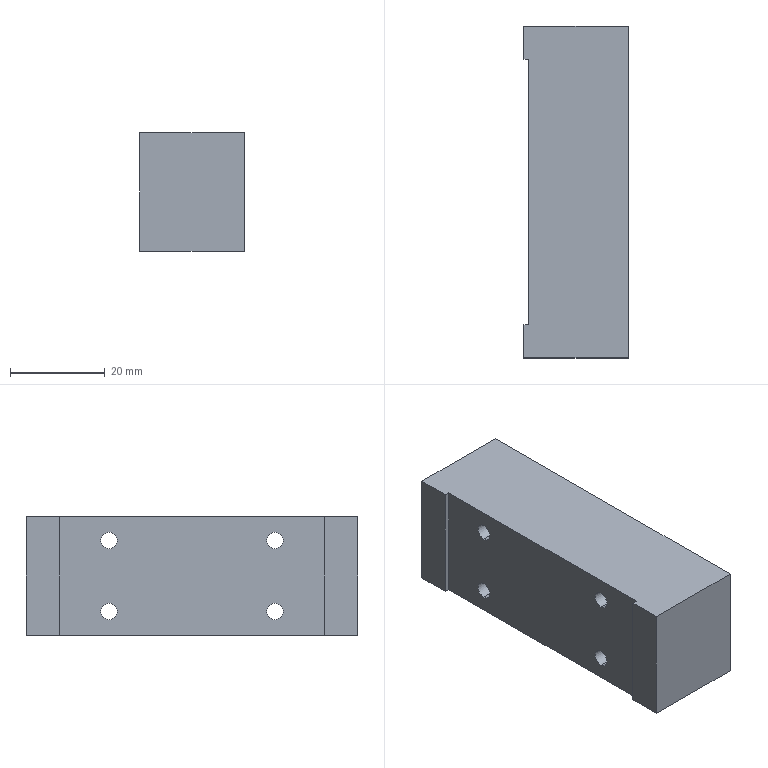Part | SolidWorks | features ICE 2, Extrusion 1 | 1 solid | 18 faces | box 22 x 70 x 25 mm | volume 36292 mm3 | plane 10 | cylinder 8 | commonest cylinder face diameters 3.5 x8
STEP:
#1=CARTESIAN_POINT('',(-10.,17.5,9.25));
#2=VERTEX_POINT('',#1);
#3=CARTESIAN_POINT('',(-10.,17.5,5.75));
#4=VERTEX_POINT('',#3);
#5=CARTESIAN_POINT('',(-10.,17.5,7.5));
#6=DIRECTION('',(1.,0.,0.));
#7=DIRECTION('',(0.,0.,1.));
#8=AXIS2_PLACEMENT_3D('',#5,#6,#7);
#9=CIRCLE('',#8,1.75);
#10=EDGE_CURVE('',#2,#4,#9,.T.);
#11=ORIENTED_EDGE('',*,*,#10,.F.);
#12=CARTESIAN_POINT('',(11.,17.5,9.25));
#13=VERTEX_POINT('',#12);
#14=CARTESIAN_POINT('',(-11.,17.5,9.25));
#15=DIRECTION('',(1.,0.,0.));
#16=VECTOR('',#15,1000.);
#17=LINE('',#14,#16);
#18=EDGE_CURVE('',#2,#13,#17,.T.);
#19=ORIENTED_EDGE('',*,*,#18,.T.);
#20=CARTESIAN_POINT('',(11.,17.5,5.75));
#21=VERTEX_POINT('',#20);
#22=CARTESIAN_POINT('',(11.,17.5,7.5));
#23=DIRECTION('',(1.,0.,0.));
#24=DIRECTION('',(0.,0.,1.));
#25=AXIS2_PLACEMENT_3D('',#22,#23,#24);
#26=CIRCLE('',#25,1.75);
#27=EDGE_CURVE('',#13,#21,#26,.T.);
#28=ORIENTED_EDGE('',*,*,#27,.T.);
#29=CARTESIAN_POINT('',(-11.,17.5,5.75));
#30=DIRECTION('',(1.,0.,0.));
#31=VECTOR('',#30,1000.);
#32=LINE('',#29,#31);
#33=EDGE_CURVE('',#4,#21,#32,.T.);
#34=ORIENTED_EDGE('',*,*,#33,.F.);
#35=EDGE_LOOP('',(#11,#19,#28,#34));
#36=FACE_OUTER_BOUND('',#35,.T.);
#37=CARTESIAN_POINT('',(-11.,17.5,7.5));
#38=DIRECTION('',(1.,0.,0.));
#39=DIRECTION('',(0.,0.,-1.));
#40=AXIS2_PLACEMENT_3D('',#37,#38,#39);
#41=CYLINDRICAL_SURFACE('',#40,1.75);
#42=ADVANCED_FACE('',(#36),#41,.F.);
#43=CARTESIAN_POINT('',(-10.,17.5,-5.75));
#44=VERTEX_POINT('',#43);
#45=CARTESIAN_POINT('',(-10.,17.5,-9.25));
#46=VERTEX_POINT('',#45);
#47=CARTESIAN_POINT('',(-10.,17.5,-7.5));
#48=DIRECTION('',(1.,0.,0.));
#49=DIRECTION('',(0.,0.,1.));
#50=AXIS2_PLACEMENT_3D('',#47,#48,#49);
#51=CIRCLE('',#50,1.75);
#52=EDGE_CURVE('',#44,#46,#51,.T.);
#53=ORIENTED_EDGE('',*,*,#52,.F.);
#54=CARTESIAN_POINT('',(11.,17.5,-5.75));
#55=VERTEX_POINT('',#54);
#56=CARTESIAN_POINT('',(-11.,17.5,-5.75));
#57=DIRECTION('',(1.,0.,0.));
#58=VECTOR('',#57,1000.);
#59=LINE('',#56,#58);
#60=EDGE_CURVE('',#44,#55,#59,.T.);
#61=ORIENTED_EDGE('',*,*,#60,.T.);
#62=CARTESIAN_POINT('',(11.,17.5,-9.25));
#63=VERTEX_POINT('',#62);
#64=CARTESIAN_POINT('',(11.,17.5,-7.5));
#65=DIRECTION('',(1.,0.,0.));
#66=DIRECTION('',(0.,0.,-1.));
#67=AXIS2_PLACEMENT_3D('',#64,#65,#66);
#68=CIRCLE('',#67,1.75);
#69=EDGE_CURVE('',#55,#63,#68,.T.);
#70=ORIENTED_EDGE('',*,*,#69,.T.);
#71=CARTESIAN_POINT('',(-11.,17.5,-9.25));
#72=DIRECTION('',(1.,0.,0.));
#73=VECTOR('',#72,1000.);
#74=LINE('',#71,#73);
#75=EDGE_CURVE('',#46,#63,#74,.T.);
#76=ORIENTED_EDGE('',*,*,#75,.F.);
#77=EDGE_LOOP('',(#53,#61,#70,#76));
#78=FACE_OUTER_BOUND('',#77,.T.);
#79=CARTESIAN_POINT('',(-11.,17.5,-7.5));
#80=DIRECTION('',(1.,0.,0.));
#81=DIRECTION('',(0.,0.,-1.));
#82=AXIS2_PLACEMENT_3D('',#79,#80,#81);
#83=CYLINDRICAL_SURFACE('',#82,1.75);
#84=ADVANCED_FACE('',(#78),#83,.F.);
#85=CARTESIAN_POINT('',(-10.,52.5,-5.75));
#86=VERTEX_POINT('',#85);
#87=CARTESIAN_POINT('',(-10.,52.5,-9.25));
#88=VERTEX_POINT('',#87);
#89=CARTESIAN_POINT('',(-10.,52.5,-7.5));
#90=DIRECTION('',(1.,0.,0.));
#91=DIRECTION('',(0.,0.,1.));
#92=AXIS2_PLACEMENT_3D('',#89,#90,#91);
#93=CIRCLE('',#92,1.75);
#94=EDGE_CURVE('',#86,#88,#93,.T.);
#95=ORIENTED_EDGE('',*,*,#94,.F.);
#96=CARTESIAN_POINT('',(11.,52.5,-5.75));
#97=VERTEX_POINT('',#96);
#98=CARTESIAN_POINT('',(-11.,52.5,-5.75));
#99=DIRECTION('',(1.,0.,0.));
#100=VECTOR('',#99,1000.);
#101=LINE('',#98,#100);
#102=EDGE_CURVE('',#86,#97,#101,.T.);
#103=ORIENTED_EDGE('',*,*,#102,.T.);
#104=CARTESIAN_POINT('',(11.,52.5,-9.25));
#105=VERTEX_POINT('',#104);
#106=CARTESIAN_POINT('',(11.,52.5,-7.5));
#107=DIRECTION('',(1.,0.,0.));
#108=DIRECTION('',(0.,0.,1.));
#109=AXIS2_PLACEMENT_3D('',#106,#107,#108);
#110=CIRCLE('',#109,1.75);
#111=EDGE_CURVE('',#97,#105,#110,.T.);
#112=ORIENTED_EDGE('',*,*,#111,.T.);
#113=CARTESIAN_POINT('',(-11.,52.5,-9.25));
#114=DIRECTION('',(1.,0.,0.));
#115=VECTOR('',#114,1000.);
#116=LINE('',#113,#115);
#117=EDGE_CURVE('',#88,#105,#116,.T.);
#118=ORIENTED_EDGE('',*,*,#117,.F.);
#119=EDGE_LOOP('',(#95,#103,#112,#118));
#120=FACE_OUTER_BOUND('',#119,.T.);
#121=CARTESIAN_POINT('',(-11.,52.5,-7.5));
#122=DIRECTION('',(1.,0.,0.));
#123=DIRECTION('',(0.,0.,-1.));
#124=AXIS2_PLACEMENT_3D('',#121,#122,#123);
#125=CYLINDRICAL_SURFACE('',#124,1.75);
#126=ADVANCED_FACE('',(#120),#125,.F.);
#127=CARTESIAN_POINT('',(-10.,52.5,9.25));
#128=VERTEX_POINT('',#127);
#129=CARTESIAN_POINT('',(-10.,52.5,5.75));
#130=VERTEX_POINT('',#129);
#131=CARTESIAN_POINT('',(-10.,52.5,7.5));
#132=DIRECTION('',(1.,0.,0.));
#133=DIRECTION('',(0.,0.,1.));
#134=AXIS2_PLACEMENT_3D('',#131,#132,#133);
#135=CIRCLE('',#134,1.75);
#136=EDGE_CURVE('',#128,#130,#135,.T.);
#137=ORIENTED_EDGE('',*,*,#136,.F.);
#138=CARTESIAN_POINT('',(11.,52.5,9.25));
#139=VERTEX_POINT('',#138);
#140=CARTESIAN_POINT('',(-11.,52.5,9.25));
#141=DIRECTION('',(1.,0.,0.));
#142=VECTOR('',#141,1000.);
#143=LINE('',#140,#142);
#144=EDGE_CURVE('',#128,#139,#143,.T.);
#145=ORIENTED_EDGE('',*,*,#144,.T.);
#146=CARTESIAN_POINT('',(11.,52.5,5.75));
#147=VERTEX_POINT('',#146);
#148=CARTESIAN_POINT('',(11.,52.5,7.5));
#149=DIRECTION('',(1.,0.,0.));
#150=DIRECTION('',(0.,0.,-1.));
#151=AXIS2_PLACEMENT_3D('',#148,#149,#150);
#152=CIRCLE('',#151,1.75);
#153=EDGE_CURVE('',#139,#147,#152,.T.);
#154=ORIENTED_EDGE('',*,*,#153,.T.);
#155=CARTESIAN_POINT('',(-11.,52.5,5.75));
#156=DIRECTION('',(1.,0.,0.));
#157=VECTOR('',#156,1000.);
#158=LINE('',#155,#157);
#159=EDGE_CURVE('',#130,#147,#158,.T.);
#160=ORIENTED_EDGE('',*,*,#159,.F.);
#161=EDGE_LOOP('',(#137,#145,#154,#160));
#162=FACE_OUTER_BOUND('',#161,.T.);
#163=CARTESIAN_POINT('',(-11.,52.5,7.5));
#164=DIRECTION('',(1.,0.,0.));
#165=DIRECTION('',(0.,0.,-1.));
#166=AXIS2_PLACEMENT_3D('',#163,#164,#165);
#167=CYLINDRICAL_SURFACE('',#166,1.75);
#168=ADVANCED_FACE('',(#162),#167,.F.);
#169=CARTESIAN_POINT('',(-11.,7.,12.5));
#170=VERTEX_POINT('',#169);
#171=CARTESIAN_POINT('',(-11.,0.,12.5));
#172=VERTEX_POINT('',#171);
#173=CARTESIAN_POINT('',(-11.,70.,12.5));
#174=DIRECTION('',(0.,-1.,0.));
#175=VECTOR('',#174,1000.);
#176=LINE('',#173,#175);
#177=EDGE_CURVE('',#170,#172,#176,.T.);
#178=ORIENTED_EDGE('',*,*,#177,.F.);
#179=CARTESIAN_POINT('',(-11.,7.,-12.5));
#180=VERTEX_POINT('',#179);
#181=CARTESIAN_POINT('',(-11.,7.,-12.5));
#182=DIRECTION('',(0.,0.,1.));
#183=VECTOR('',#182,1000.);
#184=LINE('',#181,#183);
#185=EDGE_CURVE('',#180,#170,#184,.T.);
#186=ORIENTED_EDGE('',*,*,#185,.F.);
#187=CARTESIAN_POINT('',(-11.,0.,-12.5));
#188=VERTEX_POINT('',#187);
#189=CARTESIAN_POINT('',(-11.,70.,-12.5));
#190=DIRECTION('',(0.,-1.,0.));
#191=VECTOR('',#190,1000.);
#192=LINE('',#189,#191);
#193=EDGE_CURVE('',#180,#188,#192,.T.);
#194=ORIENTED_EDGE('',*,*,#193,.T.);
#195=CARTESIAN_POINT('',(-11.,0.,-12.5));
#196=DIRECTION('',(0.,0.,1.));
#197=VECTOR('',#196,1000.);
#198=LINE('',#195,#197);
#199=EDGE_CURVE('',#188,#172,#198,.T.);
#200=ORIENTED_EDGE('',*,*,#199,.T.);
#201=EDGE_LOOP('',(#178,#186,#194,#200));
#202=FACE_OUTER_BOUND('',#201,.T.);
#203=CARTESIAN_POINT('',(-11.,70.,-12.5));
#204=DIRECTION('',(1.,0.,0.));
#205=DIRECTION('',(0.,0.,-1.));
#206=AXIS2_PLACEMENT_3D('',#203,#204,#205);
#207=PLANE('',#206);
#208=ADVANCED_FACE('',(#202),#207,.F.);
#209=ORIENTED_EDGE('',*,*,#144,.F.);
#210=CARTESIAN_POINT('',(-10.,52.5,7.5));
#211=DIRECTION('',(1.,0.,0.));
#212=DIRECTION('',(0.,0.,1.));
#213=AXIS2_PLACEMENT_3D('',#210,#211,#212);
#214=CIRCLE('',#213,1.75);
#215=EDGE_CURVE('',#130,#128,#214,.T.);
#216=ORIENTED_EDGE('',*,*,#215,.F.);
#217=ORIENTED_EDGE('',*,*,#159,.T.);
#218=CARTESIAN_POINT('',(11.,52.5,7.5));
#219=DIRECTION('',(1.,0.,0.));
#220=DIRECTION('',(0.,0.,-1.));
#221=AXIS2_PLACEMENT_3D('',#218,#219,#220);
#222=CIRCLE('',#221,1.75);
#223=EDGE_CURVE('',#147,#139,#222,.T.);
#224=ORIENTED_EDGE('',*,*,#223,.T.);
#225=EDGE_LOOP('',(#209,#216,#217,#224));
#226=FACE_OUTER_BOUND('',#225,.T.);
#227=CARTESIAN_POINT('',(-11.,52.5,7.5));
#228=DIRECTION('',(1.,0.,0.));
#229=DIRECTION('',(0.,0.,-1.));
#230=AXIS2_PLACEMENT_3D('',#227,#228,#229);
#231=CYLINDRICAL_SURFACE('',#230,1.75);
#232=ADVANCED_FACE('',(#226),#231,.F.);
#233=ORIENTED_EDGE('',*,*,#102,.F.);
#234=CARTESIAN_POINT('',(-10.,52.5,-7.5));
#235=DIRECTION('',(1.,0.,0.));
#236=DIRECTION('',(0.,0.,1.));
#237=AXIS2_PLACEMENT_3D('',#234,#235,#236);
#238=CIRCLE('',#237,1.75);
#239=EDGE_CURVE('',#88,#86,#238,.T.);
#240=ORIENTED_EDGE('',*,*,#239,.F.);
#241=ORIENTED_EDGE('',*,*,#117,.T.);
#242=CARTESIAN_POINT('',(11.,52.5,-7.5));
#243=DIRECTION('',(1.,0.,0.));
#244=DIRECTION('',(0.,0.,1.));
#245=AXIS2_PLACEMENT_3D('',#242,#243,#244);
#246=CIRCLE('',#245,1.75);
#247=EDGE_CURVE('',#105,#97,#246,.T.);
#248=ORIENTED_EDGE('',*,*,#247,.T.);
#249=EDGE_LOOP('',(#233,#240,#241,#248));
#250=FACE_OUTER_BOUND('',#249,.T.);
#251=CARTESIAN_POINT('',(-11.,52.5,-7.5));
#252=DIRECTION('',(1.,0.,0.));
#253=DIRECTION('',(0.,0.,-1.));
#254=AXIS2_PLACEMENT_3D('',#251,#252,#253);
#255=CYLINDRICAL_SURFACE('',#254,1.75);
#256=ADVANCED_FACE('',(#250),#255,.F.);
#257=ORIENTED_EDGE('',*,*,#60,.F.);
#258=CARTESIAN_POINT('',(-10.,17.5,-7.5));
#259=DIRECTION('',(1.,0.,0.));
#260=DIRECTION('',(0.,0.,1.));
#261=AXIS2_PLACEMENT_3D('',#258,#259,#260);
#262=CIRCLE('',#261,1.75);
#263=EDGE_CURVE('',#46,#44,#262,.T.);
#264=ORIENTED_EDGE('',*,*,#263,.F.);
#265=ORIENTED_EDGE('',*,*,#75,.T.);
#266=CARTESIAN_POINT('',(11.,17.5,-7.5));
#267=DIRECTION('',(1.,0.,0.));
#268=DIRECTION('',(0.,0.,-1.));
#269=AXIS2_PLACEMENT_3D('',#266,#267,#268);
#270=CIRCLE('',#269,1.75);
#271=EDGE_CURVE('',#63,#55,#270,.T.);
#272=ORIENTED_EDGE('',*,*,#271,.T.);
#273=EDGE_LOOP('',(#257,#264,#265,#272));
#274=FACE_OUTER_BOUND('',#273,.T.);
#275=CARTESIAN_POINT('',(-11.,17.5,-7.5));
#276=DIRECTION('',(1.,0.,0.));
#277=DIRECTION('',(0.,0.,-1.));
#278=AXIS2_PLACEMENT_3D('',#275,#276,#277);
#279=CYLINDRICAL_SURFACE('',#278,1.75);
#280=ADVANCED_FACE('',(#274),#279,.F.);
#281=ORIENTED_EDGE('',*,*,#18,.F.);
#282=CARTESIAN_POINT('',(-10.,17.5,7.5));
#283=DIRECTION('',(1.,0.,0.));
#284=DIRECTION('',(0.,0.,1.));
#285=AXIS2_PLACEMENT_3D('',#282,#283,#284);
#286=CIRCLE('',#285,1.75);
#287=EDGE_CURVE('',#4,#2,#286,.T.);
#288=ORIENTED_EDGE('',*,*,#287,.F.);
#289=ORIENTED_EDGE('',*,*,#33,.T.);
#290=CARTESIAN_POINT('',(11.,17.5,7.5));
#291=DIRECTION('',(1.,0.,0.));
#292=DIRECTION('',(0.,0.,1.));
#293=AXIS2_PLACEMENT_3D('',#290,#291,#292);
#294=CIRCLE('',#293,1.75);
#295=EDGE_CURVE('',#21,#13,#294,.T.);
#296=ORIENTED_EDGE('',*,*,#295,.T.);
#297=EDGE_LOOP('',(#281,#288,#289,#296));
#298=FACE_OUTER_BOUND('',#297,.T.);
#299=CARTESIAN_POINT('',(-11.,17.5,7.5));
#300=DIRECTION('',(1.,0.,0.));
#301=DIRECTION('',(0.,0.,-1.));
#302=AXIS2_PLACEMENT_3D('',#299,#300,#301);
#303=CYLINDRICAL_SURFACE('',#302,1.75);
#304=ADVANCED_FACE('',(#298),#303,.F.);
#305=ORIENTED_EDGE('',*,*,#295,.F.);
#306=ORIENTED_EDGE('',*,*,#27,.F.);
#307=EDGE_LOOP('',(#305,#306));
#308=FACE_BOUND('',#307,.T.);
#309=ORIENTED_EDGE('',*,*,#271,.F.);
#310=ORIENTED_EDGE('',*,*,#69,.F.);
#311=EDGE_LOOP('',(#309,#310));
#312=FACE_BOUND('',#311,.T.);
#313=ORIENTED_EDGE('',*,*,#247,.F.);
#314=ORIENTED_EDGE('',*,*,#111,.F.);
#315=EDGE_LOOP('',(#313,#314));
#316=FACE_BOUND('',#315,.T.);
#317=ORIENTED_EDGE('',*,*,#223,.F.);
#318=ORIENTED_EDGE('',*,*,#153,.F.);
#319=EDGE_LOOP('',(#317,#318));
#320=FACE_BOUND('',#319,.T.);
#321=CARTESIAN_POINT('',(11.,0.,12.5));
#322=VERTEX_POINT('',#321);
#323=CARTESIAN_POINT('',(11.,0.,-12.5));
#324=VERTEX_POINT('',#323);
#325=CARTESIAN_POINT('',(11.,0.,-12.5));
#326=DIRECTION('',(0.,0.,-1.));
#327=VECTOR('',#326,1000.);
#328=LINE('',#325,#327);
#329=EDGE_CURVE('',#322,#324,#328,.T.);
#330=ORIENTED_EDGE('',*,*,#329,.T.);
#331=CARTESIAN_POINT('',(11.,70.,-12.5));
#332=VERTEX_POINT('',#331);
#333=CARTESIAN_POINT('',(11.,70.,-12.5));
#334=DIRECTION('',(0.,-1.,0.));
#335=VECTOR('',#334,1000.);
#336=LINE('',#333,#335);
#337=EDGE_CURVE('',#332,#324,#336,.T.);
#338=ORIENTED_EDGE('',*,*,#337,.F.);
#339=CARTESIAN_POINT('',(11.,70.,12.5));
#340=VERTEX_POINT('',#339);
#341=CARTESIAN_POINT('',(11.,70.,-12.5));
#342=DIRECTION('',(0.,0.,-1.));
#343=VECTOR('',#342,1000.);
#344=LINE('',#341,#343);
#345=EDGE_CURVE('',#340,#332,#344,.T.);
#346=ORIENTED_EDGE('',*,*,#345,.F.);
#347=CARTESIAN_POINT('',(11.,70.,12.5));
#348=DIRECTION('',(0.,-1.,0.));
#349=VECTOR('',#348,1000.);
#350=LINE('',#347,#349);
#351=EDGE_CURVE('',#340,#322,#350,.T.);
#352=ORIENTED_EDGE('',*,*,#351,.T.);
#353=EDGE_LOOP('',(#330,#338,#346,#352));
#354=FACE_OUTER_BOUND('',#353,.T.);
#355=CARTESIAN_POINT('',(11.,70.,-12.5));
#356=DIRECTION('',(-1.,0.,0.));
#357=DIRECTION('',(0.,0.,1.));
#358=AXIS2_PLACEMENT_3D('',#355,#356,#357);
#359=PLANE('',#358);
#360=ADVANCED_FACE('',(#308,#312,#316,#320,#354),#359,.F.);
#361=ORIENTED_EDGE('',*,*,#193,.F.);
#362=CARTESIAN_POINT('',(-10.,7.,-12.5));
#363=VERTEX_POINT('',#362);
#364=CARTESIAN_POINT('',(-10.,7.,-12.5));
#365=DIRECTION('',(-1.,0.,0.));
#366=VECTOR('',#365,1000.);
#367=LINE('',#364,#366);
#368=EDGE_CURVE('',#363,#180,#367,.T.);
#369=ORIENTED_EDGE('',*,*,#368,.F.);
#370=CARTESIAN_POINT('',(-10.,63.,-12.5));
#371=VERTEX_POINT('',#370);
#372=CARTESIAN_POINT('',(-10.,63.,-12.5));
#373=DIRECTION('',(0.,-1.,0.));
#374=VECTOR('',#373,1000.);
#375=LINE('',#372,#374);
#376=EDGE_CURVE('',#371,#363,#375,.T.);
#377=ORIENTED_EDGE('',*,*,#376,.F.);
#378=CARTESIAN_POINT('',(-11.,63.,-12.5));
#379=VERTEX_POINT('',#378);
#380=CARTESIAN_POINT('',(-10.,63.,-12.5));
#381=DIRECTION('',(-1.,0.,0.));
#382=VECTOR('',#381,1000.);
#383=LINE('',#380,#382);
#384=EDGE_CURVE('',#371,#379,#383,.T.);
#385=ORIENTED_EDGE('',*,*,#384,.T.);
#386=CARTESIAN_POINT('',(-11.,70.,-12.5));
#387=VERTEX_POINT('',#386);
#388=CARTESIAN_POINT('',(-11.,70.,-12.5));
#389=DIRECTION('',(0.,-1.,0.));
#390=VECTOR('',#389,1000.);
#391=LINE('',#388,#390);
#392=EDGE_CURVE('',#387,#379,#391,.T.);
#393=ORIENTED_EDGE('',*,*,#392,.F.);
#394=CARTESIAN_POINT('',(-11.,70.,-12.5));
#395=DIRECTION('',(-1.,0.,0.));
#396=VECTOR('',#395,1000.);
#397=LINE('',#394,#396);
#398=EDGE_CURVE('',#332,#387,#397,.T.);
#399=ORIENTED_EDGE('',*,*,#398,.F.);
#400=ORIENTED_EDGE('',*,*,#337,.T.);
#401=CARTESIAN_POINT('',(-11.,0.,-12.5));
#402=DIRECTION('',(-1.,0.,0.));
#403=VECTOR('',#402,1000.);
#404=LINE('',#401,#403);
#405=EDGE_CURVE('',#324,#188,#404,.T.);
#406=ORIENTED_EDGE('',*,*,#405,.T.);
#407=EDGE_LOOP('',(#361,#369,#377,#385,#393,#399,#400,#406));
#408=FACE_OUTER_BOUND('',#407,.T.);
#409=CARTESIAN_POINT('',(-11.,70.,-12.5));
#410=DIRECTION('',(0.,0.,1.));
#411=DIRECTION('',(1.,0.,0.));
#412=AXIS2_PLACEMENT_3D('',#409,#410,#411);
#413=PLANE('',#412);
#414=ADVANCED_FACE('',(#408),#413,.F.);
#415=ORIENTED_EDGE('',*,*,#392,.T.);
#416=CARTESIAN_POINT('',(-11.,63.,12.5));
#417=VERTEX_POINT('',#416);
#418=CARTESIAN_POINT('',(-11.,63.,-12.5));
#419=DIRECTION('',(0.,0.,-1.));
#420=VECTOR('',#419,1000.);
#421=LINE('',#418,#420);
#422=EDGE_CURVE('',#417,#379,#421,.T.);
#423=ORIENTED_EDGE('',*,*,#422,.F.);
#424=CARTESIAN_POINT('',(-11.,70.,12.5));
#425=VERTEX_POINT('',#424);
#426=CARTESIAN_POINT('',(-11.,70.,12.5));
#427=DIRECTION('',(0.,-1.,0.));
#428=VECTOR('',#427,1000.);
#429=LINE('',#426,#428);
#430=EDGE_CURVE('',#425,#417,#429,.T.);
#431=ORIENTED_EDGE('',*,*,#430,.F.);
#432=CARTESIAN_POINT('',(-11.,70.,-12.5));
#433=DIRECTION('',(0.,0.,1.));
#434=VECTOR('',#433,1000.);
#435=LINE('',#432,#434);
#436=EDGE_CURVE('',#387,#425,#435,.T.);
#437=ORIENTED_EDGE('',*,*,#436,.F.);
#438=EDGE_LOOP('',(#415,#423,#431,#437));
#439=FACE_OUTER_BOUND('',#438,.T.);
#440=CARTESIAN_POINT('',(-11.,70.,-12.5));
#441=DIRECTION('',(1.,0.,0.));
#442=DIRECTION('',(0.,0.,-1.));
#443=AXIS2_PLACEMENT_3D('',#440,#441,#442);
#444=PLANE('',#443);
#445=ADVANCED_FACE('',(#439),#444,.F.);
#446=CARTESIAN_POINT('',(-10.,7.,12.5));
#447=VERTEX_POINT('',#446);
#448=CARTESIAN_POINT('',(-10.,63.,12.5));
#449=VERTEX_POINT('',#448);
#450=CARTESIAN_POINT('',(-10.,63.,12.5));
#451=DIRECTION('',(0.,1.,0.));
#452=VECTOR('',#451,1000.);
#453=LINE('',#450,#452);
#454=EDGE_CURVE('',#447,#449,#453,.T.);
#455=ORIENTED_EDGE('',*,*,#454,.F.);
#456=CARTESIAN_POINT('',(-10.,7.,12.5));
#457=DIRECTION('',(-1.,0.,0.));
#458=VECTOR('',#457,1000.);
#459=LINE('',#456,#458);
#460=EDGE_CURVE('',#447,#170,#459,.T.);
#461=ORIENTED_EDGE('',*,*,#460,.T.);
#462=ORIENTED_EDGE('',*,*,#177,.T.);
#463=CARTESIAN_POINT('',(-11.,0.,12.5));
#464=DIRECTION('',(1.,0.,0.));
#465=VECTOR('',#464,1000.);
#466=LINE('',#463,#465);
#467=EDGE_CURVE('',#172,#322,#466,.T.);
#468=ORIENTED_EDGE('',*,*,#467,.T.);
#469=ORIENTED_EDGE('',*,*,#351,.F.);
#470=CARTESIAN_POINT('',(-11.,70.,12.5));
#471=DIRECTION('',(1.,0.,0.));
#472=VECTOR('',#471,1000.);
#473=LINE('',#470,#472);
#474=EDGE_CURVE('',#425,#340,#473,.T.);
#475=ORIENTED_EDGE('',*,*,#474,.F.);
#476=ORIENTED_EDGE('',*,*,#430,.T.);
#477=CARTESIAN_POINT('',(-10.,63.,12.5));
#478=DIRECTION('',(-1.,0.,0.));
#479=VECTOR('',#478,1000.);
#480=LINE('',#477,#479);
#481=EDGE_CURVE('',#449,#417,#480,.T.);
#482=ORIENTED_EDGE('',*,*,#481,.F.);
#483=EDGE_LOOP('',(#455,#461,#462,#468,#469,#475,#476,#482));
#484=FACE_OUTER_BOUND('',#483,.T.);
#485=CARTESIAN_POINT('',(-11.,70.,12.5));
#486=DIRECTION('',(0.,0.,-1.));
#487=DIRECTION('',(-1.,0.,0.));
#488=AXIS2_PLACEMENT_3D('',#485,#486,#487);
#489=PLANE('',#488);
#490=ADVANCED_FACE('',(#484),#489,.F.);
#491=ORIENTED_EDGE('',*,*,#345,.T.);
#492=ORIENTED_EDGE('',*,*,#398,.T.);
#493=ORIENTED_EDGE('',*,*,#436,.T.);
#494=ORIENTED_EDGE('',*,*,#474,.T.);
#495=EDGE_LOOP('',(#491,#492,#493,#494));
#496=FACE_OUTER_BOUND('',#495,.T.);
#497=CARTESIAN_POINT('',(0.,70.,0.));
#498=DIRECTION('',(0.,1.,0.));
#499=DIRECTION('',(0.,0.,1.));
#500=AXIS2_PLACEMENT_3D('',#497,#498,#499);
#501=PLANE('',#500);
#502=ADVANCED_FACE('',(#496),#501,.T.);
#503=ORIENTED_EDGE('',*,*,#329,.F.);
#504=ORIENTED_EDGE('',*,*,#467,.F.);
#505=ORIENTED_EDGE('',*,*,#199,.F.);
#506=ORIENTED_EDGE('',*,*,#405,.F.);
#507=EDGE_LOOP('',(#503,#504,#505,#506));
#508=FACE_OUTER_BOUND('',#507,.T.);
#509=CARTESIAN_POINT('',(0.,0.,0.));
#510=DIRECTION('',(0.,1.,0.));
#511=DIRECTION('',(0.,0.,1.));
#512=AXIS2_PLACEMENT_3D('',#509,#510,#511);
#513=PLANE('',#512);
#514=ADVANCED_FACE('',(#508),#513,.F.);
#515=ORIENTED_EDGE('',*,*,#239,.T.);
#516=ORIENTED_EDGE('',*,*,#94,.T.);
#517=EDGE_LOOP('',(#515,#516));
#518=FACE_BOUND('',#517,.T.);
#519=ORIENTED_EDGE('',*,*,#287,.T.);
#520=ORIENTED_EDGE('',*,*,#10,.T.);
#521=EDGE_LOOP('',(#519,#520));
#522=FACE_BOUND('',#521,.T.);
#523=ORIENTED_EDGE('',*,*,#454,.T.);
#524=CARTESIAN_POINT('',(-10.,63.,-12.5));
#525=DIRECTION('',(0.,0.,-1.));
#526=VECTOR('',#525,1000.);
#527=LINE('',#524,#526);
#528=EDGE_CURVE('',#449,#371,#527,.T.);
#529=ORIENTED_EDGE('',*,*,#528,.T.);
#530=ORIENTED_EDGE('',*,*,#376,.T.);
#531=CARTESIAN_POINT('',(-10.,7.,-12.5));
#532=DIRECTION('',(0.,0.,1.));
#533=VECTOR('',#532,1000.);
#534=LINE('',#531,#533);
#535=EDGE_CURVE('',#363,#447,#534,.T.);
#536=ORIENTED_EDGE('',*,*,#535,.T.);
#537=EDGE_LOOP('',(#523,#529,#530,#536));
#538=FACE_OUTER_BOUND('',#537,.T.);
#539=ORIENTED_EDGE('',*,*,#263,.T.);
#540=ORIENTED_EDGE('',*,*,#52,.T.);
#541=EDGE_LOOP('',(#539,#540));
#542=FACE_BOUND('',#541,.T.);
#543=ORIENTED_EDGE('',*,*,#215,.T.);
#544=ORIENTED_EDGE('',*,*,#136,.T.);
#545=EDGE_LOOP('',(#543,#544));
#546=FACE_BOUND('',#545,.T.);
#547=CARTESIAN_POINT('',(-10.,0.,0.));
#548=DIRECTION('',(-1.,0.,0.));
#549=DIRECTION('',(0.,0.,1.));
#550=AXIS2_PLACEMENT_3D('',#547,#548,#549);
#551=PLANE('',#550);
#552=ADVANCED_FACE('',(#518,#522,#538,#542,#546),#551,.T.);
#553=ORIENTED_EDGE('',*,*,#185,.T.);
#554=ORIENTED_EDGE('',*,*,#460,.F.);
#555=ORIENTED_EDGE('',*,*,#535,.F.);
#556=ORIENTED_EDGE('',*,*,#368,.T.);
#557=EDGE_LOOP('',(#553,#554,#555,#556));
#558=FACE_OUTER_BOUND('',#557,.T.);
#559=CARTESIAN_POINT('',(-10.,7.,-12.5));
#560=DIRECTION('',(0.,-1.,0.));
#561=DIRECTION('',(0.,0.,-1.));
#562=AXIS2_PLACEMENT_3D('',#559,#560,#561);
#563=PLANE('',#562);
#564=ADVANCED_FACE('',(#558),#563,.F.);
#565=ORIENTED_EDGE('',*,*,#422,.T.);
#566=ORIENTED_EDGE('',*,*,#384,.F.);
#567=ORIENTED_EDGE('',*,*,#528,.F.);
#568=ORIENTED_EDGE('',*,*,#481,.T.);
#569=EDGE_LOOP('',(#565,#566,#567,#568));
#570=FACE_OUTER_BOUND('',#569,.T.);
#571=CARTESIAN_POINT('',(-10.,63.,-12.5));
#572=DIRECTION('',(0.,1.,0.));
#573=DIRECTION('',(0.,0.,1.));
#574=AXIS2_PLACEMENT_3D('',#571,#572,#573);
#575=PLANE('',#574);
#576=ADVANCED_FACE('',(#570),#575,.F.);
#577=CLOSED_SHELL('',(#42,#84,#126,#168,#208,#232,#256,#280,#304,#360,#414,#445,#490,#502,#514,#552,#564,#576));
#578=MANIFOLD_SOLID_BREP('',#577);
#579=CARTESIAN_POINT('',(0.,0.,0.));
#580=DIRECTION('',(0.,0.,1.));
#581=DIRECTION('',(1.,0.,0.));
#582=AXIS2_PLACEMENT_3D('',#579,#580,#581);
#583=(LENGTH_UNIT()NAMED_UNIT(*)SI_UNIT(.MILLI.,.METRE.));
#584=UNCERTAINTY_MEASURE_WITH_UNIT(LENGTH_MEASURE(0.00001),#583,'','');
#585=(NAMED_UNIT(*)PLANE_ANGLE_UNIT()SI_UNIT($,.RADIAN.));
#586=(NAMED_UNIT(*)SI_UNIT($,.STERADIAN.)SOLID_ANGLE_UNIT());
#587=(GEOMETRIC_REPRESENTATION_CONTEXT(3)GLOBAL_UNCERTAINTY_ASSIGNED_CONTEXT((#584))GLOBAL_UNIT_ASSIGNED_CONTEXT((#583,#585,#586))REPRESENTATION_CONTEXT('',''));
#588=ADVANCED_BREP_SHAPE_REPRESENTATION('',(#578,#582),#587);